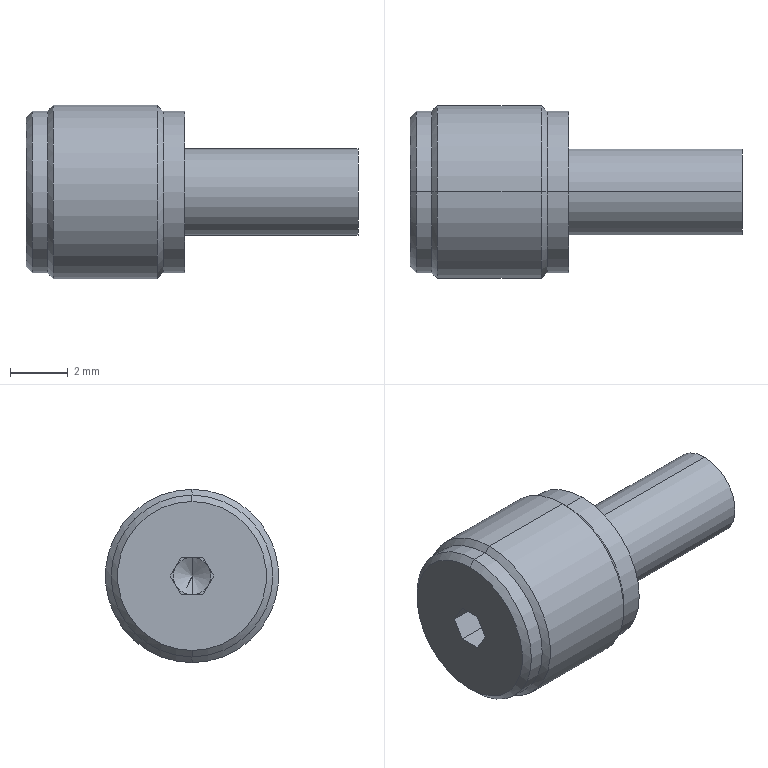Part | SolidWorks | features BaseBody 1 | 1 solid | 31 faces | box 11.5 x 6 x 6 mm | volume 188.495 mm3 | plane 15 | cylinder 8 | cone 8 | commonest cylinder face diameters 5.6 x4 3 x2 6 x2
STEP:
#1=CARTESIAN_POINT('',(6.,0.,1.5));
#2=VERTEX_POINT('',#1);
#3=CARTESIAN_POINT('',(6.,0.,-1.5));
#4=VERTEX_POINT('',#3);
#5=CARTESIAN_POINT('',(6.,0.,0.));
#6=DIRECTION('',(-1.,0.,0.));
#7=DIRECTION('',(0.,0.,1.));
#8=AXIS2_PLACEMENT_3D('',#5,#6,#7);
#9=CIRCLE('',#8,1.5);
#10=EDGE_CURVE('',#2,#4,#9,.T.);
#11=ORIENTED_EDGE('',*,*,#10,.T.);
#12=CARTESIAN_POINT('',(0.,0.,-1.5));
#13=VERTEX_POINT('',#12);
#14=CARTESIAN_POINT('',(-4.975,0.,-1.5));
#15=DIRECTION('',(-1.,0.,0.));
#16=VECTOR('',#15,1000.);
#17=LINE('',#14,#16);
#18=EDGE_CURVE('',#4,#13,#17,.T.);
#19=ORIENTED_EDGE('',*,*,#18,.T.);
#20=CARTESIAN_POINT('',(0.,0.,1.5));
#21=VERTEX_POINT('',#20);
#22=CARTESIAN_POINT('',(0.,0.,0.));
#23=DIRECTION('',(-1.,0.,0.));
#24=DIRECTION('',(0.,0.,1.));
#25=AXIS2_PLACEMENT_3D('',#22,#23,#24);
#26=CIRCLE('',#25,1.5);
#27=EDGE_CURVE('',#21,#13,#26,.T.);
#28=ORIENTED_EDGE('',*,*,#27,.F.);
#29=CARTESIAN_POINT('',(-4.975,0.,1.5));
#30=DIRECTION('',(-1.,0.,0.));
#31=VECTOR('',#30,1000.);
#32=LINE('',#29,#31);
#33=EDGE_CURVE('',#2,#21,#32,.T.);
#34=ORIENTED_EDGE('',*,*,#33,.F.);
#35=EDGE_LOOP('',(#11,#19,#28,#34));
#36=FACE_OUTER_BOUND('',#35,.T.);
#37=CARTESIAN_POINT('',(-4.975,0.,0.));
#38=DIRECTION('',(-1.,0.,0.));
#39=DIRECTION('',(0.,0.,1.));
#40=AXIS2_PLACEMENT_3D('',#37,#38,#39);
#41=CYLINDRICAL_SURFACE('',#40,1.5);
#42=ADVANCED_FACE('',(#36),#41,.T.);
#43=CARTESIAN_POINT('',(0.,0.,2.8));
#44=VERTEX_POINT('',#43);
#45=CARTESIAN_POINT('',(0.,0.,-2.8));
#46=VERTEX_POINT('',#45);
#47=CARTESIAN_POINT('',(0.,0.,0.));
#48=DIRECTION('',(-1.,0.,0.));
#49=DIRECTION('',(0.,0.,1.));
#50=AXIS2_PLACEMENT_3D('',#47,#48,#49);
#51=CIRCLE('',#50,2.8);
#52=EDGE_CURVE('',#44,#46,#51,.T.);
#53=ORIENTED_EDGE('',*,*,#52,.T.);
#54=CARTESIAN_POINT('',(-0.75,0.,-2.8));
#55=VERTEX_POINT('',#54);
#56=CARTESIAN_POINT('',(-4.975,0.,-2.8));
#57=DIRECTION('',(-1.,0.,0.));
#58=VECTOR('',#57,1000.);
#59=LINE('',#56,#58);
#60=EDGE_CURVE('',#46,#55,#59,.T.);
#61=ORIENTED_EDGE('',*,*,#60,.T.);
#62=CARTESIAN_POINT('',(-0.75,0.,2.8));
#63=VERTEX_POINT('',#62);
#64=CARTESIAN_POINT('',(-0.75,0.,0.));
#65=DIRECTION('',(-1.,0.,0.));
#66=DIRECTION('',(0.,0.,1.));
#67=AXIS2_PLACEMENT_3D('',#64,#65,#66);
#68=CIRCLE('',#67,2.8);
#69=EDGE_CURVE('',#63,#55,#68,.T.);
#70=ORIENTED_EDGE('',*,*,#69,.F.);
#71=CARTESIAN_POINT('',(-4.975,0.,2.8));
#72=DIRECTION('',(-1.,0.,0.));
#73=VECTOR('',#72,1000.);
#74=LINE('',#71,#73);
#75=EDGE_CURVE('',#44,#63,#74,.T.);
#76=ORIENTED_EDGE('',*,*,#75,.F.);
#77=EDGE_LOOP('',(#53,#61,#70,#76));
#78=FACE_OUTER_BOUND('',#77,.T.);
#79=CARTESIAN_POINT('',(-4.975,0.,0.));
#80=DIRECTION('',(-1.,0.,0.));
#81=DIRECTION('',(0.,0.,1.));
#82=AXIS2_PLACEMENT_3D('',#79,#80,#81);
#83=CYLINDRICAL_SURFACE('',#82,2.8);
#84=ADVANCED_FACE('',(#78),#83,.T.);
#85=ORIENTED_EDGE('',*,*,#69,.T.);
#86=CARTESIAN_POINT('',(-0.95,0.,-3.));
#87=VERTEX_POINT('',#86);
#88=CARTESIAN_POINT('',(-0.75,0.,-2.8));
#89=DIRECTION('',(-0.7071,0.,-0.7071));
#90=VECTOR('',#89,1000.);
#91=LINE('',#88,#90);
#92=EDGE_CURVE('',#55,#87,#91,.T.);
#93=ORIENTED_EDGE('',*,*,#92,.T.);
#94=CARTESIAN_POINT('',(-0.95,0.,3.));
#95=VERTEX_POINT('',#94);
#96=CARTESIAN_POINT('',(-0.95,0.,0.));
#97=DIRECTION('',(-1.,0.,0.));
#98=DIRECTION('',(0.,0.,1.));
#99=AXIS2_PLACEMENT_3D('',#96,#97,#98);
#100=CIRCLE('',#99,3.);
#101=EDGE_CURVE('',#95,#87,#100,.T.);
#102=ORIENTED_EDGE('',*,*,#101,.F.);
#103=CARTESIAN_POINT('',(-0.75,0.,2.8));
#104=DIRECTION('',(-0.7071,0.,0.7071));
#105=VECTOR('',#104,1000.);
#106=LINE('',#103,#105);
#107=EDGE_CURVE('',#63,#95,#106,.T.);
#108=ORIENTED_EDGE('',*,*,#107,.F.);
#109=EDGE_LOOP('',(#85,#93,#102,#108));
#110=FACE_OUTER_BOUND('',#109,.T.);
#111=CARTESIAN_POINT('',(-0.75,0.,0.));
#112=DIRECTION('',(-1.,0.,0.));
#113=DIRECTION('',(0.,0.,1.));
#114=AXIS2_PLACEMENT_3D('',#111,#112,#113);
#115=CONICAL_SURFACE('',#114,2.8,0.7854);
#116=ADVANCED_FACE('',(#110),#115,.T.);
#117=ORIENTED_EDGE('',*,*,#101,.T.);
#118=CARTESIAN_POINT('',(-4.55,0.,-3.));
#119=VERTEX_POINT('',#118);
#120=CARTESIAN_POINT('',(-4.975,0.,-3.));
#121=DIRECTION('',(-1.,0.,0.));
#122=VECTOR('',#121,1000.);
#123=LINE('',#120,#122);
#124=EDGE_CURVE('',#87,#119,#123,.T.);
#125=ORIENTED_EDGE('',*,*,#124,.T.);
#126=CARTESIAN_POINT('',(-4.55,0.,3.));
#127=VERTEX_POINT('',#126);
#128=CARTESIAN_POINT('',(-4.55,0.,0.));
#129=DIRECTION('',(-1.,0.,0.));
#130=DIRECTION('',(0.,0.,1.));
#131=AXIS2_PLACEMENT_3D('',#128,#129,#130);
#132=CIRCLE('',#131,3.);
#133=EDGE_CURVE('',#127,#119,#132,.T.);
#134=ORIENTED_EDGE('',*,*,#133,.F.);
#135=CARTESIAN_POINT('',(-4.975,0.,3.));
#136=DIRECTION('',(-1.,0.,0.));
#137=VECTOR('',#136,1000.);
#138=LINE('',#135,#137);
#139=EDGE_CURVE('',#95,#127,#138,.T.);
#140=ORIENTED_EDGE('',*,*,#139,.F.);
#141=EDGE_LOOP('',(#117,#125,#134,#140));
#142=FACE_OUTER_BOUND('',#141,.T.);
#143=CARTESIAN_POINT('',(-4.975,0.,0.));
#144=DIRECTION('',(-1.,0.,0.));
#145=DIRECTION('',(0.,0.,1.));
#146=AXIS2_PLACEMENT_3D('',#143,#144,#145);
#147=CYLINDRICAL_SURFACE('',#146,3.);
#148=ADVANCED_FACE('',(#142),#147,.T.);
#149=CARTESIAN_POINT('',(-4.75,0.,2.8));
#150=VERTEX_POINT('',#149);
#151=CARTESIAN_POINT('',(-4.75,0.,-2.8));
#152=VERTEX_POINT('',#151);
#153=CARTESIAN_POINT('',(-4.75,0.,0.));
#154=DIRECTION('',(-1.,0.,0.));
#155=DIRECTION('',(0.,0.,1.));
#156=AXIS2_PLACEMENT_3D('',#153,#154,#155);
#157=CIRCLE('',#156,2.8);
#158=EDGE_CURVE('',#150,#152,#157,.T.);
#159=ORIENTED_EDGE('',*,*,#158,.F.);
#160=CARTESIAN_POINT('',(-4.55,0.,3.));
#161=DIRECTION('',(0.7071,0.,0.7071));
#162=VECTOR('',#161,1000.);
#163=LINE('',#160,#162);
#164=EDGE_CURVE('',#150,#127,#163,.T.);
#165=ORIENTED_EDGE('',*,*,#164,.T.);
#166=ORIENTED_EDGE('',*,*,#133,.T.);
#167=CARTESIAN_POINT('',(-4.55,0.,-3.));
#168=DIRECTION('',(0.7071,0.,-0.7071));
#169=VECTOR('',#168,1000.);
#170=LINE('',#167,#169);
#171=EDGE_CURVE('',#152,#119,#170,.T.);
#172=ORIENTED_EDGE('',*,*,#171,.F.);
#173=EDGE_LOOP('',(#159,#165,#166,#172));
#174=FACE_OUTER_BOUND('',#173,.T.);
#175=CARTESIAN_POINT('',(-4.55,0.,0.));
#176=DIRECTION('',(1.,0.,0.));
#177=DIRECTION('',(0.,0.,-1.));
#178=AXIS2_PLACEMENT_3D('',#175,#176,#177);
#179=CONICAL_SURFACE('',#178,3.,0.7854);
#180=ADVANCED_FACE('',(#174),#179,.T.);
#181=ORIENTED_EDGE('',*,*,#158,.T.);
#182=CARTESIAN_POINT('',(-5.28,0.,-2.8));
#183=VERTEX_POINT('',#182);
#184=CARTESIAN_POINT('',(-4.975,0.,-2.8));
#185=DIRECTION('',(-1.,0.,0.));
#186=VECTOR('',#185,1000.);
#187=LINE('',#184,#186);
#188=EDGE_CURVE('',#152,#183,#187,.T.);
#189=ORIENTED_EDGE('',*,*,#188,.T.);
#190=CARTESIAN_POINT('',(-5.28,0.,2.8));
#191=VERTEX_POINT('',#190);
#192=CARTESIAN_POINT('',(-5.28,0.,0.));
#193=DIRECTION('',(-1.,0.,0.));
#194=DIRECTION('',(0.,0.,1.));
#195=AXIS2_PLACEMENT_3D('',#192,#193,#194);
#196=CIRCLE('',#195,2.8);
#197=EDGE_CURVE('',#191,#183,#196,.T.);
#198=ORIENTED_EDGE('',*,*,#197,.F.);
#199=CARTESIAN_POINT('',(-4.975,0.,2.8));
#200=DIRECTION('',(-1.,0.,0.));
#201=VECTOR('',#200,1000.);
#202=LINE('',#199,#201);
#203=EDGE_CURVE('',#150,#191,#202,.T.);
#204=ORIENTED_EDGE('',*,*,#203,.F.);
#205=EDGE_LOOP('',(#181,#189,#198,#204));
#206=FACE_OUTER_BOUND('',#205,.T.);
#207=CARTESIAN_POINT('',(-4.975,0.,0.));
#208=DIRECTION('',(-1.,0.,0.));
#209=DIRECTION('',(0.,0.,1.));
#210=AXIS2_PLACEMENT_3D('',#207,#208,#209);
#211=CYLINDRICAL_SURFACE('',#210,2.8);
#212=ADVANCED_FACE('',(#206),#211,.T.);
#213=CARTESIAN_POINT('',(-5.5,0.,2.58));
#214=VERTEX_POINT('',#213);
#215=CARTESIAN_POINT('',(-5.5,0.,-2.58));
#216=VERTEX_POINT('',#215);
#217=CARTESIAN_POINT('',(-5.5,0.,0.));
#218=DIRECTION('',(-1.,0.,0.));
#219=DIRECTION('',(0.,0.,1.));
#220=AXIS2_PLACEMENT_3D('',#217,#218,#219);
#221=CIRCLE('',#220,2.58);
#222=EDGE_CURVE('',#214,#216,#221,.T.);
#223=ORIENTED_EDGE('',*,*,#222,.F.);
#224=CARTESIAN_POINT('',(-5.28,0.,2.8));
#225=DIRECTION('',(0.7071,0.,0.7071));
#226=VECTOR('',#225,1000.);
#227=LINE('',#224,#226);
#228=EDGE_CURVE('',#214,#191,#227,.T.);
#229=ORIENTED_EDGE('',*,*,#228,.T.);
#230=ORIENTED_EDGE('',*,*,#197,.T.);
#231=CARTESIAN_POINT('',(-5.28,0.,-2.8));
#232=DIRECTION('',(0.7071,0.,-0.7071));
#233=VECTOR('',#232,1000.);
#234=LINE('',#231,#233);
#235=EDGE_CURVE('',#216,#183,#234,.T.);
#236=ORIENTED_EDGE('',*,*,#235,.F.);
#237=EDGE_LOOP('',(#223,#229,#230,#236));
#238=FACE_OUTER_BOUND('',#237,.T.);
#239=CARTESIAN_POINT('',(-5.28,0.,0.));
#240=DIRECTION('',(1.,0.,0.));
#241=DIRECTION('',(0.,0.,-1.));
#242=AXIS2_PLACEMENT_3D('',#239,#240,#241);
#243=CONICAL_SURFACE('',#242,2.8,0.7854);
#244=ADVANCED_FACE('',(#238),#243,.T.);
#245=CARTESIAN_POINT('',(-3.309,0.,0.));
#246=VERTEX_POINT('',#245);
#247=CARTESIAN_POINT('',(-3.7,0.,0.65));
#248=VERTEX_POINT('',#247);
#249=CARTESIAN_POINT('',(-1003.309,0.,1664.279));
#250=DIRECTION('',(-0.515,0.,0.8572));
#251=VECTOR('',#250,1000.);
#252=LINE('',#249,#251);
#253=EDGE_CURVE('',#246,#248,#252,.T.);
#254=ORIENTED_EDGE('',*,*,#253,.F.);
#255=CARTESIAN_POINT('',(-3.7,0.,-0.65));
#256=VERTEX_POINT('',#255);
#257=CARTESIAN_POINT('',(-1003.309,0.,-1664.279));
#258=DIRECTION('',(-0.515,0.,-0.8572));
#259=VECTOR('',#258,1000.);
#260=LINE('',#257,#259);
#261=EDGE_CURVE('',#246,#256,#260,.T.);
#262=ORIENTED_EDGE('',*,*,#261,.T.);
#263=CARTESIAN_POINT('',(-3.7,-0.5629,-0.325));
#264=VERTEX_POINT('',#263);
#265=CARTESIAN_POINT('',(-3.7,0.,0.));
#266=DIRECTION('',(-1.,0.,0.));
#267=DIRECTION('',(0.,0.,1.));
#268=AXIS2_PLACEMENT_3D('',#265,#266,#267);
#269=CIRCLE('',#268,0.65);
#270=EDGE_CURVE('',#256,#264,#269,.T.);
#271=ORIENTED_EDGE('',*,*,#270,.T.);
#272=CARTESIAN_POINT('',(-3.7,-0.5629,0.325));
#273=VERTEX_POINT('',#272);
#274=CARTESIAN_POINT('',(-3.7,0.,0.));
#275=DIRECTION('',(-1.,0.,0.));
#276=DIRECTION('',(0.,0.,1.));
#277=AXIS2_PLACEMENT_3D('',#274,#275,#276);
#278=CIRCLE('',#277,0.65);
#279=EDGE_CURVE('',#264,#273,#278,.T.);
#280=ORIENTED_EDGE('',*,*,#279,.T.);
#281=CARTESIAN_POINT('',(-3.7,0.,0.));
#282=DIRECTION('',(-1.,0.,0.));
#283=DIRECTION('',(0.,0.,1.));
#284=AXIS2_PLACEMENT_3D('',#281,#282,#283);
#285=CIRCLE('',#284,0.65);
#286=EDGE_CURVE('',#273,#248,#285,.T.);
#287=ORIENTED_EDGE('',*,*,#286,.T.);
#288=EDGE_LOOP('',(#254,#262,#271,#280,#287));
#289=FACE_OUTER_BOUND('',#288,.T.);
#290=CARTESIAN_POINT('',(-1003.309,0.,0.));
#291=DIRECTION('',(-1.,0.,0.));
#292=DIRECTION('',(0.,0.,1.));
#293=AXIS2_PLACEMENT_3D('',#290,#291,#292);
#294=CONICAL_SURFACE('',#293,1664.279,1.03);
#295=ADVANCED_FACE('',(#289),#294,.F.);
#296=ORIENTED_EDGE('',*,*,#261,.F.);
#297=ORIENTED_EDGE('',*,*,#253,.T.);
#298=CARTESIAN_POINT('',(-3.7,0.5629,0.325));
#299=VERTEX_POINT('',#298);
#300=CARTESIAN_POINT('',(-3.7,0.,0.));
#301=DIRECTION('',(-1.,0.,0.));
#302=DIRECTION('',(0.,0.,1.));
#303=AXIS2_PLACEMENT_3D('',#300,#301,#302);
#304=CIRCLE('',#303,0.65);
#305=EDGE_CURVE('',#248,#299,#304,.T.);
#306=ORIENTED_EDGE('',*,*,#305,.T.);
#307=CARTESIAN_POINT('',(-3.7,0.5629,-0.325));
#308=VERTEX_POINT('',#307);
#309=CARTESIAN_POINT('',(-3.7,0.,0.));
#310=DIRECTION('',(-1.,0.,0.));
#311=DIRECTION('',(0.,0.,1.));
#312=AXIS2_PLACEMENT_3D('',#309,#310,#311);
#313=CIRCLE('',#312,0.65);
#314=EDGE_CURVE('',#299,#308,#313,.T.);
#315=ORIENTED_EDGE('',*,*,#314,.T.);
#316=CARTESIAN_POINT('',(-3.7,0.,0.));
#317=DIRECTION('',(-1.,0.,0.));
#318=DIRECTION('',(0.,0.,1.));
#319=AXIS2_PLACEMENT_3D('',#316,#317,#318);
#320=CIRCLE('',#319,0.65);
#321=EDGE_CURVE('',#308,#256,#320,.T.);
#322=ORIENTED_EDGE('',*,*,#321,.T.);
#323=EDGE_LOOP('',(#296,#297,#306,#315,#322));
#324=FACE_OUTER_BOUND('',#323,.T.);
#325=CARTESIAN_POINT('',(-1003.309,0.,0.));
#326=DIRECTION('',(-1.,0.,0.));
#327=DIRECTION('',(0.,0.,1.));
#328=AXIS2_PLACEMENT_3D('',#325,#326,#327);
#329=CONICAL_SURFACE('',#328,1664.279,1.03);
#330=ADVANCED_FACE('',(#324),#329,.F.);
#331=ORIENTED_EDGE('',*,*,#270,.F.);
#332=CARTESIAN_POINT('',(-3.7,-0.3753,-0.65));
#333=VERTEX_POINT('',#332);
#334=CARTESIAN_POINT('',(-3.7,-0.3753,-0.65));
#335=DIRECTION('',(0.,1.,0.));
#336=VECTOR('',#335,1000.);
#337=LINE('',#334,#336);
#338=EDGE_CURVE('',#333,#256,#337,.T.);
#339=ORIENTED_EDGE('',*,*,#338,.F.);
#340=CARTESIAN_POINT('',(-3.7,-0.7506,0.));
#341=DIRECTION('',(0.,0.5,-0.866));
#342=VECTOR('',#341,1000.);
#343=LINE('',#340,#342);
#344=EDGE_CURVE('',#264,#333,#343,.T.);
#345=ORIENTED_EDGE('',*,*,#344,.F.);
#346=EDGE_LOOP('',(#331,#339,#345));
#347=FACE_OUTER_BOUND('',#346,.T.);
#348=CARTESIAN_POINT('',(-3.7,0.,0.));
#349=DIRECTION('',(1.,0.,0.));
#350=DIRECTION('',(0.,1.,0.));
#351=AXIS2_PLACEMENT_3D('',#348,#349,#350);
#352=PLANE('',#351);
#353=ADVANCED_FACE('',(#347),#352,.F.);
#354=ORIENTED_EDGE('',*,*,#279,.F.);
#355=CARTESIAN_POINT('',(-3.7,-0.7506,0.));
#356=VERTEX_POINT('',#355);
#357=CARTESIAN_POINT('',(-3.7,-0.7506,0.));
#358=DIRECTION('',(0.,0.5,-0.866));
#359=VECTOR('',#358,1000.);
#360=LINE('',#357,#359);
#361=EDGE_CURVE('',#356,#264,#360,.T.);
#362=ORIENTED_EDGE('',*,*,#361,.F.);
#363=CARTESIAN_POINT('',(-3.7,-0.3753,0.65));
#364=DIRECTION('',(0.,-0.5,-0.866));
#365=VECTOR('',#364,1000.);
#366=LINE('',#363,#365);
#367=EDGE_CURVE('',#273,#356,#366,.T.);
#368=ORIENTED_EDGE('',*,*,#367,.F.);
#369=EDGE_LOOP('',(#354,#362,#368));
#370=FACE_OUTER_BOUND('',#369,.T.);
#371=CARTESIAN_POINT('',(-3.7,0.,0.));
#372=DIRECTION('',(1.,0.,0.));
#373=DIRECTION('',(0.,1.,0.));
#374=AXIS2_PLACEMENT_3D('',#371,#372,#373);
#375=PLANE('',#374);
#376=ADVANCED_FACE('',(#370),#375,.F.);
#377=ORIENTED_EDGE('',*,*,#286,.F.);
#378=CARTESIAN_POINT('',(-3.7,-0.3753,0.65));
#379=VERTEX_POINT('',#378);
#380=CARTESIAN_POINT('',(-3.7,-0.3753,0.65));
#381=DIRECTION('',(0.,-0.5,-0.866));
#382=VECTOR('',#381,1000.);
#383=LINE('',#380,#382);
#384=EDGE_CURVE('',#379,#273,#383,.T.);
#385=ORIENTED_EDGE('',*,*,#384,.F.);
#386=CARTESIAN_POINT('',(-3.7,0.3753,0.65));
#387=DIRECTION('',(0.,-1.,0.));
#388=VECTOR('',#387,1000.);
#389=LINE('',#386,#388);
#390=EDGE_CURVE('',#248,#379,#389,.T.);
#391=ORIENTED_EDGE('',*,*,#390,.F.);
#392=EDGE_LOOP('',(#377,#385,#391));
#393=FACE_OUTER_BOUND('',#392,.T.);
#394=CARTESIAN_POINT('',(-3.7,0.,0.));
#395=DIRECTION('',(1.,0.,0.));
#396=DIRECTION('',(0.,1.,0.));
#397=AXIS2_PLACEMENT_3D('',#394,#395,#396);
#398=PLANE('',#397);
#399=ADVANCED_FACE('',(#393),#398,.F.);
#400=ORIENTED_EDGE('',*,*,#305,.F.);
#401=CARTESIAN_POINT('',(-3.7,0.3753,0.65));
#402=VERTEX_POINT('',#401);
#403=CARTESIAN_POINT('',(-3.7,0.3753,0.65));
#404=DIRECTION('',(0.,-1.,0.));
#405=VECTOR('',#404,1000.);
#406=LINE('',#403,#405);
#407=EDGE_CURVE('',#402,#248,#406,.T.);
#408=ORIENTED_EDGE('',*,*,#407,.F.);
#409=CARTESIAN_POINT('',(-3.7,0.7506,0.));
#410=DIRECTION('',(0.,-0.5,0.866));
#411=VECTOR('',#410,1000.);
#412=LINE('',#409,#411);
#413=EDGE_CURVE('',#299,#402,#412,.T.);
#414=ORIENTED_EDGE('',*,*,#413,.F.);
#415=EDGE_LOOP('',(#400,#408,#414));
#416=FACE_OUTER_BOUND('',#415,.T.);
#417=CARTESIAN_POINT('',(-3.7,0.,0.));
#418=DIRECTION('',(1.,0.,0.));
#419=DIRECTION('',(0.,1.,0.));
#420=AXIS2_PLACEMENT_3D('',#417,#418,#419);
#421=PLANE('',#420);
#422=ADVANCED_FACE('',(#416),#421,.F.);
#423=ORIENTED_EDGE('',*,*,#314,.F.);
#424=CARTESIAN_POINT('',(-3.7,0.7506,0.));
#425=VERTEX_POINT('',#424);
#426=CARTESIAN_POINT('',(-3.7,0.7506,0.));
#427=DIRECTION('',(0.,-0.5,0.866));
#428=VECTOR('',#427,1000.);
#429=LINE('',#426,#428);
#430=EDGE_CURVE('',#425,#299,#429,.T.);
#431=ORIENTED_EDGE('',*,*,#430,.F.);
#432=CARTESIAN_POINT('',(-3.7,0.3753,-0.65));
#433=DIRECTION('',(0.,0.5,0.866));
#434=VECTOR('',#433,1000.);
#435=LINE('',#432,#434);
#436=EDGE_CURVE('',#308,#425,#435,.T.);
#437=ORIENTED_EDGE('',*,*,#436,.F.);
#438=EDGE_LOOP('',(#423,#431,#437));
#439=FACE_OUTER_BOUND('',#438,.T.);
#440=CARTESIAN_POINT('',(-3.7,0.,0.));
#441=DIRECTION('',(1.,0.,0.));
#442=DIRECTION('',(0.,1.,0.));
#443=AXIS2_PLACEMENT_3D('',#440,#441,#442);
#444=PLANE('',#443);
#445=ADVANCED_FACE('',(#439),#444,.F.);
#446=ORIENTED_EDGE('',*,*,#321,.F.);
#447=CARTESIAN_POINT('',(-3.7,0.3753,-0.65));
#448=VERTEX_POINT('',#447);
#449=CARTESIAN_POINT('',(-3.7,0.3753,-0.65));
#450=DIRECTION('',(0.,0.5,0.866));
#451=VECTOR('',#450,1000.);
#452=LINE('',#449,#451);
#453=EDGE_CURVE('',#448,#308,#452,.T.);
#454=ORIENTED_EDGE('',*,*,#453,.F.);
#455=CARTESIAN_POINT('',(-3.7,-0.3753,-0.65));
#456=DIRECTION('',(0.,1.,0.));
#457=VECTOR('',#456,1000.);
#458=LINE('',#455,#457);
#459=EDGE_CURVE('',#256,#448,#458,.T.);
#460=ORIENTED_EDGE('',*,*,#459,.F.);
#461=EDGE_LOOP('',(#446,#454,#460));
#462=FACE_OUTER_BOUND('',#461,.T.);
#463=CARTESIAN_POINT('',(-3.7,0.,0.));
#464=DIRECTION('',(1.,0.,0.));
#465=DIRECTION('',(0.,1.,0.));
#466=AXIS2_PLACEMENT_3D('',#463,#464,#465);
#467=PLANE('',#466);
#468=ADVANCED_FACE('',(#462),#467,.F.);
#469=ORIENTED_EDGE('',*,*,#338,.T.);
#470=ORIENTED_EDGE('',*,*,#459,.T.);
#471=CARTESIAN_POINT('',(-5.5,0.3753,-0.65));
#472=VERTEX_POINT('',#471);
#473=CARTESIAN_POINT('',(-3.7,0.3753,-0.65));
#474=DIRECTION('',(-1.,0.,0.));
#475=VECTOR('',#474,1000.);
#476=LINE('',#473,#475);
#477=EDGE_CURVE('',#448,#472,#476,.T.);
#478=ORIENTED_EDGE('',*,*,#477,.T.);
#479=CARTESIAN_POINT('',(-5.5,-0.3753,-0.65));
#480=VERTEX_POINT('',#479);
#481=CARTESIAN_POINT('',(-5.5,-0.3753,-0.65));
#482=DIRECTION('',(0.,1.,0.));
#483=VECTOR('',#482,1000.);
#484=LINE('',#481,#483);
#485=EDGE_CURVE('',#480,#472,#484,.T.);
#486=ORIENTED_EDGE('',*,*,#485,.F.);
#487=CARTESIAN_POINT('',(-3.7,-0.3753,-0.65));
#488=DIRECTION('',(-1.,0.,0.));
#489=VECTOR('',#488,1000.);
#490=LINE('',#487,#489);
#491=EDGE_CURVE('',#333,#480,#490,.T.);
#492=ORIENTED_EDGE('',*,*,#491,.F.);
#493=EDGE_LOOP('',(#469,#470,#478,#486,#492));
#494=FACE_OUTER_BOUND('',#493,.T.);
#495=CARTESIAN_POINT('',(-3.7,-0.3753,-0.65));
#496=DIRECTION('',(0.,0.,1.));
#497=DIRECTION('',(1.,0.,0.));
#498=AXIS2_PLACEMENT_3D('',#495,#496,#497);
#499=PLANE('',#498);
#500=ADVANCED_FACE('',(#494),#499,.T.);
#501=ORIENTED_EDGE('',*,*,#361,.T.);
#502=ORIENTED_EDGE('',*,*,#344,.T.);
#503=ORIENTED_EDGE('',*,*,#491,.T.);
#504=CARTESIAN_POINT('',(-5.5,-0.7506,0.));
#505=VERTEX_POINT('',#504);
#506=CARTESIAN_POINT('',(-5.5,-0.7506,0.));
#507=DIRECTION('',(0.,0.5,-0.866));
#508=VECTOR('',#507,1000.);
#509=LINE('',#506,#508);
#510=EDGE_CURVE('',#505,#480,#509,.T.);
#511=ORIENTED_EDGE('',*,*,#510,.F.);
#512=CARTESIAN_POINT('',(-3.7,-0.7506,0.));
#513=DIRECTION('',(-1.,0.,0.));
#514=VECTOR('',#513,1000.);
#515=LINE('',#512,#514);
#516=EDGE_CURVE('',#356,#505,#515,.T.);
#517=ORIENTED_EDGE('',*,*,#516,.F.);
#518=EDGE_LOOP('',(#501,#502,#503,#511,#517));
#519=FACE_OUTER_BOUND('',#518,.T.);
#520=CARTESIAN_POINT('',(-3.7,-0.7506,0.));
#521=DIRECTION('',(0.,0.866,0.5));
#522=DIRECTION('',(1.,0.,0.));
#523=AXIS2_PLACEMENT_3D('',#520,#521,#522);
#524=PLANE('',#523);
#525=ADVANCED_FACE('',(#519),#524,.T.);
#526=ORIENTED_EDGE('',*,*,#384,.T.);
#527=ORIENTED_EDGE('',*,*,#367,.T.);
#528=ORIENTED_EDGE('',*,*,#516,.T.);
#529=CARTESIAN_POINT('',(-5.5,-0.3753,0.65));
#530=VERTEX_POINT('',#529);
#531=CARTESIAN_POINT('',(-5.5,-0.3753,0.65));
#532=DIRECTION('',(0.,-0.5,-0.866));
#533=VECTOR('',#532,1000.);
#534=LINE('',#531,#533);
#535=EDGE_CURVE('',#530,#505,#534,.T.);
#536=ORIENTED_EDGE('',*,*,#535,.F.);
#537=CARTESIAN_POINT('',(-3.7,-0.3753,0.65));
#538=DIRECTION('',(-1.,0.,0.));
#539=VECTOR('',#538,1000.);
#540=LINE('',#537,#539);
#541=EDGE_CURVE('',#379,#530,#540,.T.);
#542=ORIENTED_EDGE('',*,*,#541,.F.);
#543=EDGE_LOOP('',(#526,#527,#528,#536,#542));
#544=FACE_OUTER_BOUND('',#543,.T.);
#545=CARTESIAN_POINT('',(-3.7,-0.3753,0.65));
#546=DIRECTION('',(0.,0.866,-0.5));
#547=DIRECTION('',(-1.,0.,0.));
#548=AXIS2_PLACEMENT_3D('',#545,#546,#547);
#549=PLANE('',#548);
#550=ADVANCED_FACE('',(#544),#549,.T.);
#551=ORIENTED_EDGE('',*,*,#407,.T.);
#552=ORIENTED_EDGE('',*,*,#390,.T.);
#553=ORIENTED_EDGE('',*,*,#541,.T.);
#554=CARTESIAN_POINT('',(-5.5,0.3753,0.65));
#555=VERTEX_POINT('',#554);
#556=CARTESIAN_POINT('',(-5.5,0.3753,0.65));
#557=DIRECTION('',(0.,-1.,0.));
#558=VECTOR('',#557,1000.);
#559=LINE('',#556,#558);
#560=EDGE_CURVE('',#555,#530,#559,.T.);
#561=ORIENTED_EDGE('',*,*,#560,.F.);
#562=CARTESIAN_POINT('',(-3.7,0.3753,0.65));
#563=DIRECTION('',(-1.,0.,0.));
#564=VECTOR('',#563,1000.);
#565=LINE('',#562,#564);
#566=EDGE_CURVE('',#402,#555,#565,.T.);
#567=ORIENTED_EDGE('',*,*,#566,.F.);
#568=EDGE_LOOP('',(#551,#552,#553,#561,#567));
#569=FACE_OUTER_BOUND('',#568,.T.);
#570=CARTESIAN_POINT('',(-3.7,0.3753,0.65));
#571=DIRECTION('',(0.,0.,-1.));
#572=DIRECTION('',(0.,-1.,0.));
#573=AXIS2_PLACEMENT_3D('',#570,#571,#572);
#574=PLANE('',#573);
#575=ADVANCED_FACE('',(#569),#574,.T.);
#576=ORIENTED_EDGE('',*,*,#430,.T.);
#577=ORIENTED_EDGE('',*,*,#413,.T.);
#578=ORIENTED_EDGE('',*,*,#566,.T.);
#579=CARTESIAN_POINT('',(-5.5,0.7506,0.));
#580=VERTEX_POINT('',#579);
#581=CARTESIAN_POINT('',(-5.5,0.7506,0.));
#582=DIRECTION('',(0.,-0.5,0.866));
#583=VECTOR('',#582,1000.);
#584=LINE('',#581,#583);
#585=EDGE_CURVE('',#580,#555,#584,.T.);
#586=ORIENTED_EDGE('',*,*,#585,.F.);
#587=CARTESIAN_POINT('',(-3.7,0.7506,0.));
#588=DIRECTION('',(-1.,0.,0.));
#589=VECTOR('',#588,1000.);
#590=LINE('',#587,#589);
#591=EDGE_CURVE('',#425,#580,#590,.T.);
#592=ORIENTED_EDGE('',*,*,#591,.F.);
#593=EDGE_LOOP('',(#576,#577,#578,#586,#592));
#594=FACE_OUTER_BOUND('',#593,.T.);
#595=CARTESIAN_POINT('',(-3.7,0.7506,0.));
#596=DIRECTION('',(0.,-0.866,-0.5));
#597=DIRECTION('',(0.,0.5,-0.866));
#598=AXIS2_PLACEMENT_3D('',#595,#596,#597);
#599=PLANE('',#598);
#600=ADVANCED_FACE('',(#594),#599,.T.);
#601=ORIENTED_EDGE('',*,*,#453,.T.);
#602=ORIENTED_EDGE('',*,*,#436,.T.);
#603=ORIENTED_EDGE('',*,*,#591,.T.);
#604=CARTESIAN_POINT('',(-5.5,0.3753,-0.65));
#605=DIRECTION('',(0.,0.5,0.866));
#606=VECTOR('',#605,1000.);
#607=LINE('',#604,#606);
#608=EDGE_CURVE('',#472,#580,#607,.T.);
#609=ORIENTED_EDGE('',*,*,#608,.F.);
#610=ORIENTED_EDGE('',*,*,#477,.F.);
#611=EDGE_LOOP('',(#601,#602,#603,#609,#610));
#612=FACE_OUTER_BOUND('',#611,.T.);
#613=CARTESIAN_POINT('',(-3.7,0.3753,-0.65));
#614=DIRECTION('',(0.,-0.866,0.5));
#615=DIRECTION('',(-1.,0.,0.));
#616=AXIS2_PLACEMENT_3D('',#613,#614,#615);
#617=PLANE('',#616);
#618=ADVANCED_FACE('',(#612),#617,.T.);
#619=ORIENTED_EDGE('',*,*,#228,.F.);
#620=CARTESIAN_POINT('',(-5.5,0.,0.));
#621=DIRECTION('',(-1.,0.,0.));
#622=DIRECTION('',(0.,0.,1.));
#623=AXIS2_PLACEMENT_3D('',#620,#621,#622);
#624=CIRCLE('',#623,2.58);
#625=EDGE_CURVE('',#216,#214,#624,.T.);
#626=ORIENTED_EDGE('',*,*,#625,.F.);
#627=ORIENTED_EDGE('',*,*,#235,.T.);
#628=CARTESIAN_POINT('',(-5.28,0.,0.));
#629=DIRECTION('',(-1.,0.,0.));
#630=DIRECTION('',(0.,0.,1.));
#631=AXIS2_PLACEMENT_3D('',#628,#629,#630);
#632=CIRCLE('',#631,2.8);
#633=EDGE_CURVE('',#183,#191,#632,.T.);
#634=ORIENTED_EDGE('',*,*,#633,.T.);
#635=EDGE_LOOP('',(#619,#626,#627,#634));
#636=FACE_OUTER_BOUND('',#635,.T.);
#637=CARTESIAN_POINT('',(-5.28,0.,0.));
#638=DIRECTION('',(1.,0.,0.));
#639=DIRECTION('',(0.,0.,-1.));
#640=AXIS2_PLACEMENT_3D('',#637,#638,#639);
#641=CONICAL_SURFACE('',#640,2.8,0.7854);
#642=ADVANCED_FACE('',(#636),#641,.T.);
#643=ORIENTED_EDGE('',*,*,#188,.F.);
#644=CARTESIAN_POINT('',(-4.75,0.,0.));
#645=DIRECTION('',(-1.,0.,0.));
#646=DIRECTION('',(0.,0.,1.));
#647=AXIS2_PLACEMENT_3D('',#644,#645,#646);
#648=CIRCLE('',#647,2.8);
#649=EDGE_CURVE('',#152,#150,#648,.T.);
#650=ORIENTED_EDGE('',*,*,#649,.T.);
#651=ORIENTED_EDGE('',*,*,#203,.T.);
#652=ORIENTED_EDGE('',*,*,#633,.F.);
#653=EDGE_LOOP('',(#643,#650,#651,#652));
#654=FACE_OUTER_BOUND('',#653,.T.);
#655=CARTESIAN_POINT('',(-4.975,0.,0.));
#656=DIRECTION('',(-1.,0.,0.));
#657=DIRECTION('',(0.,0.,1.));
#658=AXIS2_PLACEMENT_3D('',#655,#656,#657);
#659=CYLINDRICAL_SURFACE('',#658,2.8);
#660=ADVANCED_FACE('',(#654),#659,.T.);
#661=ORIENTED_EDGE('',*,*,#164,.F.);
#662=ORIENTED_EDGE('',*,*,#649,.F.);
#663=ORIENTED_EDGE('',*,*,#171,.T.);
#664=CARTESIAN_POINT('',(-4.55,0.,0.));
#665=DIRECTION('',(-1.,0.,0.));
#666=DIRECTION('',(0.,0.,1.));
#667=AXIS2_PLACEMENT_3D('',#664,#665,#666);
#668=CIRCLE('',#667,3.);
#669=EDGE_CURVE('',#119,#127,#668,.T.);
#670=ORIENTED_EDGE('',*,*,#669,.T.);
#671=EDGE_LOOP('',(#661,#662,#663,#670));
#672=FACE_OUTER_BOUND('',#671,.T.);
#673=CARTESIAN_POINT('',(-4.55,0.,0.));
#674=DIRECTION('',(1.,0.,0.));
#675=DIRECTION('',(0.,0.,-1.));
#676=AXIS2_PLACEMENT_3D('',#673,#674,#675);
#677=CONICAL_SURFACE('',#676,3.,0.7854);
#678=ADVANCED_FACE('',(#672),#677,.T.);
#679=ORIENTED_EDGE('',*,*,#124,.F.);
#680=CARTESIAN_POINT('',(-0.95,0.,0.));
#681=DIRECTION('',(-1.,0.,0.));
#682=DIRECTION('',(0.,0.,1.));
#683=AXIS2_PLACEMENT_3D('',#680,#681,#682);
#684=CIRCLE('',#683,3.);
#685=EDGE_CURVE('',#87,#95,#684,.T.);
#686=ORIENTED_EDGE('',*,*,#685,.T.);
#687=ORIENTED_EDGE('',*,*,#139,.T.);
#688=ORIENTED_EDGE('',*,*,#669,.F.);
#689=EDGE_LOOP('',(#679,#686,#687,#688));
#690=FACE_OUTER_BOUND('',#689,.T.);
#691=CARTESIAN_POINT('',(-4.975,0.,0.));
#692=DIRECTION('',(-1.,0.,0.));
#693=DIRECTION('',(0.,0.,1.));
#694=AXIS2_PLACEMENT_3D('',#691,#692,#693);
#695=CYLINDRICAL_SURFACE('',#694,3.);
#696=ADVANCED_FACE('',(#690),#695,.T.);
#697=ORIENTED_EDGE('',*,*,#92,.F.);
#698=CARTESIAN_POINT('',(-0.75,0.,0.));
#699=DIRECTION('',(-1.,0.,0.));
#700=DIRECTION('',(0.,0.,1.));
#701=AXIS2_PLACEMENT_3D('',#698,#699,#700);
#702=CIRCLE('',#701,2.8);
#703=EDGE_CURVE('',#55,#63,#702,.T.);
#704=ORIENTED_EDGE('',*,*,#703,.T.);
#705=ORIENTED_EDGE('',*,*,#107,.T.);
#706=ORIENTED_EDGE('',*,*,#685,.F.);
#707=EDGE_LOOP('',(#697,#704,#705,#706));
#708=FACE_OUTER_BOUND('',#707,.T.);
#709=CARTESIAN_POINT('',(-0.75,0.,0.));
#710=DIRECTION('',(-1.,0.,0.));
#711=DIRECTION('',(0.,0.,1.));
#712=AXIS2_PLACEMENT_3D('',#709,#710,#711);
#713=CONICAL_SURFACE('',#712,2.8,0.7854);
#714=ADVANCED_FACE('',(#708),#713,.T.);
#715=ORIENTED_EDGE('',*,*,#60,.F.);
#716=CARTESIAN_POINT('',(0.,0.,0.));
#717=DIRECTION('',(-1.,0.,0.));
#718=DIRECTION('',(0.,0.,1.));
#719=AXIS2_PLACEMENT_3D('',#716,#717,#718);
#720=CIRCLE('',#719,2.8);
#721=EDGE_CURVE('',#46,#44,#720,.T.);
#722=ORIENTED_EDGE('',*,*,#721,.T.);
#723=ORIENTED_EDGE('',*,*,#75,.T.);
#724=ORIENTED_EDGE('',*,*,#703,.F.);
#725=EDGE_LOOP('',(#715,#722,#723,#724));
#726=FACE_OUTER_BOUND('',#725,.T.);
#727=CARTESIAN_POINT('',(-4.975,0.,0.));
#728=DIRECTION('',(-1.,0.,0.));
#729=DIRECTION('',(0.,0.,1.));
#730=AXIS2_PLACEMENT_3D('',#727,#728,#729);
#731=CYLINDRICAL_SURFACE('',#730,2.8);
#732=ADVANCED_FACE('',(#726),#731,.T.);
#733=ORIENTED_EDGE('',*,*,#27,.T.);
#734=CARTESIAN_POINT('',(0.,0.,0.));
#735=DIRECTION('',(-1.,0.,0.));
#736=DIRECTION('',(0.,0.,1.));
#737=AXIS2_PLACEMENT_3D('',#734,#735,#736);
#738=CIRCLE('',#737,1.5);
#739=EDGE_CURVE('',#13,#21,#738,.T.);
#740=ORIENTED_EDGE('',*,*,#739,.T.);
#741=EDGE_LOOP('',(#733,#740));
#742=FACE_BOUND('',#741,.T.);
#743=ORIENTED_EDGE('',*,*,#52,.F.);
#744=ORIENTED_EDGE('',*,*,#721,.F.);
#745=EDGE_LOOP('',(#743,#744));
#746=FACE_OUTER_BOUND('',#745,.T.);
#747=CARTESIAN_POINT('',(0.,2.8,0.));
#748=DIRECTION('',(-1.,0.,0.));
#749=DIRECTION('',(0.,0.,1.));
#750=AXIS2_PLACEMENT_3D('',#747,#748,#749);
#751=PLANE('',#750);
#752=ADVANCED_FACE('',(#742,#746),#751,.F.);
#753=ORIENTED_EDGE('',*,*,#18,.F.);
#754=CARTESIAN_POINT('',(6.,0.,0.));
#755=DIRECTION('',(-1.,0.,0.));
#756=DIRECTION('',(0.,0.,1.));
#757=AXIS2_PLACEMENT_3D('',#754,#755,#756);
#758=CIRCLE('',#757,1.5);
#759=EDGE_CURVE('',#4,#2,#758,.T.);
#760=ORIENTED_EDGE('',*,*,#759,.T.);
#761=ORIENTED_EDGE('',*,*,#33,.T.);
#762=ORIENTED_EDGE('',*,*,#739,.F.);
#763=EDGE_LOOP('',(#753,#760,#761,#762));
#764=FACE_OUTER_BOUND('',#763,.T.);
#765=CARTESIAN_POINT('',(-4.975,0.,0.));
#766=DIRECTION('',(-1.,0.,0.));
#767=DIRECTION('',(0.,0.,1.));
#768=AXIS2_PLACEMENT_3D('',#765,#766,#767);
#769=CYLINDRICAL_SURFACE('',#768,1.5);
#770=ADVANCED_FACE('',(#764),#769,.T.);
#771=ORIENTED_EDGE('',*,*,#10,.F.);
#772=ORIENTED_EDGE('',*,*,#759,.F.);
#773=EDGE_LOOP('',(#771,#772));
#774=FACE_OUTER_BOUND('',#773,.T.);
#775=CARTESIAN_POINT('',(6.,1.5,0.));
#776=DIRECTION('',(-1.,0.,0.));
#777=DIRECTION('',(0.,0.,1.));
#778=AXIS2_PLACEMENT_3D('',#775,#776,#777);
#779=PLANE('',#778);
#780=ADVANCED_FACE('',(#774),#779,.F.);
#781=ORIENTED_EDGE('',*,*,#560,.T.);
#782=ORIENTED_EDGE('',*,*,#535,.T.);
#783=ORIENTED_EDGE('',*,*,#510,.T.);
#784=ORIENTED_EDGE('',*,*,#485,.T.);
#785=ORIENTED_EDGE('',*,*,#608,.T.);
#786=ORIENTED_EDGE('',*,*,#585,.T.);
#787=EDGE_LOOP('',(#781,#782,#783,#784,#785,#786));
#788=FACE_BOUND('',#787,.T.);
#789=ORIENTED_EDGE('',*,*,#625,.T.);
#790=ORIENTED_EDGE('',*,*,#222,.T.);
#791=EDGE_LOOP('',(#789,#790));
#792=FACE_OUTER_BOUND('',#791,.T.);
#793=CARTESIAN_POINT('',(-5.5,2.58,0.));
#794=DIRECTION('',(1.,0.,0.));
#795=DIRECTION('',(0.,1.,0.));
#796=AXIS2_PLACEMENT_3D('',#793,#794,#795);
#797=PLANE('',#796);
#798=ADVANCED_FACE('',(#788,#792),#797,.F.);
#799=CLOSED_SHELL('',(#42,#84,#116,#148,#180,#212,#244,#295,#330,#353,#376,#399,#422,#445,#468,#500,#525,#550,#575,#600,#618,#642,#660,#678,#696,#714,#732,#752,#770,#780,#798));
#800=MANIFOLD_SOLID_BREP('',#799);
#801=CARTESIAN_POINT('',(0.,0.,0.));
#802=DIRECTION('',(0.,0.,1.));
#803=DIRECTION('',(1.,0.,0.));
#804=AXIS2_PLACEMENT_3D('',#801,#802,#803);
#805=(LENGTH_UNIT()NAMED_UNIT(*)SI_UNIT(.MILLI.,.METRE.));
#806=UNCERTAINTY_MEASURE_WITH_UNIT(LENGTH_MEASURE(0.00001),#805,'','');
#807=(NAMED_UNIT(*)PLANE_ANGLE_UNIT()SI_UNIT($,.RADIAN.));
#808=(NAMED_UNIT(*)SI_UNIT($,.STERADIAN.)SOLID_ANGLE_UNIT());
#809=(GEOMETRIC_REPRESENTATION_CONTEXT(3)GLOBAL_UNCERTAINTY_ASSIGNED_CONTEXT((#806))GLOBAL_UNIT_ASSIGNED_CONTEXT((#805,#807,#808))REPRESENTATION_CONTEXT('',''));
#810=ADVANCED_BREP_SHAPE_REPRESENTATION('',(#800,#804),#809);